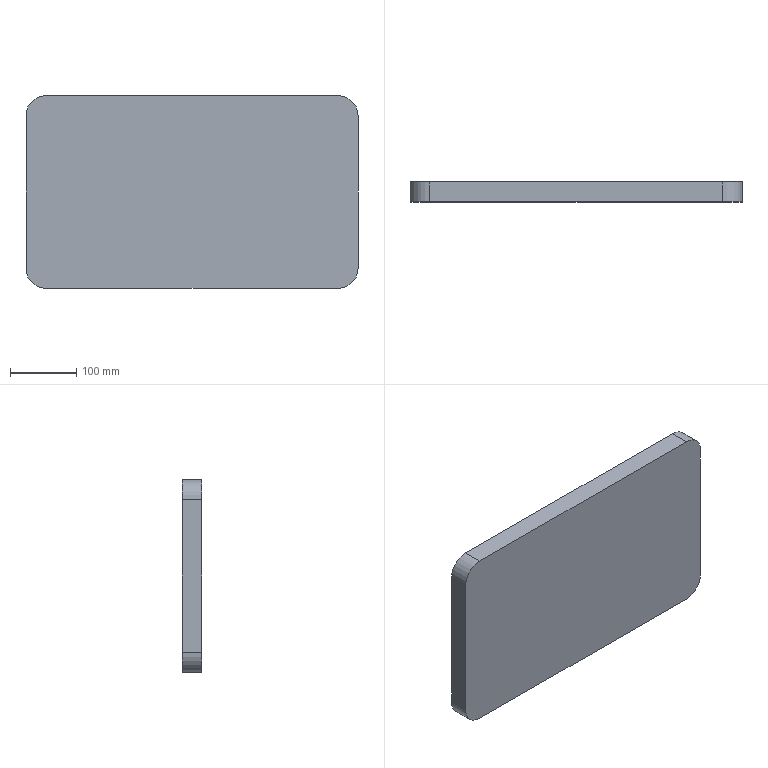Part | SolidWorks | features Extrusion 1, ICE 1 | 1 solid | 19 faces | box 500 x 30 x 290 mm | volume 838737 mm3 | plane 11 | cylinder 8 | commonest cylinder face diameters 60 x8
STEP:
#1=CARTESIAN_POINT('',(250.,0.,-115.));
#2=VERTEX_POINT('',#1);
#3=CARTESIAN_POINT('',(220.,0.,-145.));
#4=VERTEX_POINT('',#3);
#5=CARTESIAN_POINT('',(220.,0.,-115.));
#6=DIRECTION('',(0.,1.,0.));
#7=DIRECTION('',(0.,0.,1.));
#8=AXIS2_PLACEMENT_3D('',#5,#6,#7);
#9=CIRCLE('',#8,30.);
#10=EDGE_CURVE('',#2,#4,#9,.T.);
#11=ORIENTED_EDGE('',*,*,#10,.T.);
#12=CARTESIAN_POINT('',(220.,30.,-145.));
#13=VERTEX_POINT('',#12);
#14=CARTESIAN_POINT('',(220.,30.,-145.));
#15=DIRECTION('',(0.,-1.,0.));
#16=VECTOR('',#15,1000.);
#17=LINE('',#14,#16);
#18=EDGE_CURVE('',#13,#4,#17,.T.);
#19=ORIENTED_EDGE('',*,*,#18,.F.);
#20=CARTESIAN_POINT('',(250.,30.,-115.));
#21=VERTEX_POINT('',#20);
#22=CARTESIAN_POINT('',(220.,30.,-115.));
#23=DIRECTION('',(0.,1.,0.));
#24=DIRECTION('',(0.,0.,1.));
#25=AXIS2_PLACEMENT_3D('',#22,#23,#24);
#26=CIRCLE('',#25,30.);
#27=EDGE_CURVE('',#21,#13,#26,.T.);
#28=ORIENTED_EDGE('',*,*,#27,.F.);
#29=CARTESIAN_POINT('',(250.,30.,-115.));
#30=DIRECTION('',(0.,-1.,0.));
#31=VECTOR('',#30,1000.);
#32=LINE('',#29,#31);
#33=EDGE_CURVE('',#21,#2,#32,.T.);
#34=ORIENTED_EDGE('',*,*,#33,.T.);
#35=EDGE_LOOP('',(#11,#19,#28,#34));
#36=FACE_OUTER_BOUND('',#35,.T.);
#37=CARTESIAN_POINT('',(220.,30.,-115.));
#38=DIRECTION('',(0.,-1.,0.));
#39=DIRECTION('',(0.,0.,-1.));
#40=AXIS2_PLACEMENT_3D('',#37,#38,#39);
#41=CYLINDRICAL_SURFACE('',#40,30.);
#42=ADVANCED_FACE('',(#36),#41,.T.);
#43=CARTESIAN_POINT('',(-220.,0.,-145.));
#44=VERTEX_POINT('',#43);
#45=CARTESIAN_POINT('',(-220.,0.,-145.));
#46=DIRECTION('',(-1.,0.,0.));
#47=VECTOR('',#46,1000.);
#48=LINE('',#45,#47);
#49=EDGE_CURVE('',#4,#44,#48,.T.);
#50=ORIENTED_EDGE('',*,*,#49,.T.);
#51=CARTESIAN_POINT('',(-220.,30.,-145.));
#52=VERTEX_POINT('',#51);
#53=CARTESIAN_POINT('',(-220.,30.,-145.));
#54=DIRECTION('',(0.,-1.,0.));
#55=VECTOR('',#54,1000.);
#56=LINE('',#53,#55);
#57=EDGE_CURVE('',#52,#44,#56,.T.);
#58=ORIENTED_EDGE('',*,*,#57,.F.);
#59=CARTESIAN_POINT('',(-220.,30.,-145.));
#60=DIRECTION('',(-1.,0.,0.));
#61=VECTOR('',#60,1000.);
#62=LINE('',#59,#61);
#63=EDGE_CURVE('',#13,#52,#62,.T.);
#64=ORIENTED_EDGE('',*,*,#63,.F.);
#65=ORIENTED_EDGE('',*,*,#18,.T.);
#66=EDGE_LOOP('',(#50,#58,#64,#65));
#67=FACE_OUTER_BOUND('',#66,.T.);
#68=CARTESIAN_POINT('',(-220.,30.,-145.));
#69=DIRECTION('',(0.,0.,1.));
#70=DIRECTION('',(1.,0.,0.));
#71=AXIS2_PLACEMENT_3D('',#68,#69,#70);
#72=PLANE('',#71);
#73=ADVANCED_FACE('',(#67),#72,.F.);
#74=CARTESIAN_POINT('',(-250.,0.,-115.));
#75=VERTEX_POINT('',#74);
#76=CARTESIAN_POINT('',(-220.,0.,-115.));
#77=DIRECTION('',(0.,1.,0.));
#78=DIRECTION('',(0.,0.,-1.));
#79=AXIS2_PLACEMENT_3D('',#76,#77,#78);
#80=CIRCLE('',#79,30.);
#81=EDGE_CURVE('',#44,#75,#80,.T.);
#82=ORIENTED_EDGE('',*,*,#81,.T.);
#83=CARTESIAN_POINT('',(-250.,30.,-115.));
#84=VERTEX_POINT('',#83);
#85=CARTESIAN_POINT('',(-250.,30.,-115.));
#86=DIRECTION('',(0.,-1.,0.));
#87=VECTOR('',#86,1000.);
#88=LINE('',#85,#87);
#89=EDGE_CURVE('',#84,#75,#88,.T.);
#90=ORIENTED_EDGE('',*,*,#89,.F.);
#91=CARTESIAN_POINT('',(-220.,30.,-115.));
#92=DIRECTION('',(0.,1.,0.));
#93=DIRECTION('',(0.,0.,-1.));
#94=AXIS2_PLACEMENT_3D('',#91,#92,#93);
#95=CIRCLE('',#94,30.);
#96=EDGE_CURVE('',#52,#84,#95,.T.);
#97=ORIENTED_EDGE('',*,*,#96,.F.);
#98=ORIENTED_EDGE('',*,*,#57,.T.);
#99=EDGE_LOOP('',(#82,#90,#97,#98));
#100=FACE_OUTER_BOUND('',#99,.T.);
#101=CARTESIAN_POINT('',(-220.,30.,-115.));
#102=DIRECTION('',(0.,-1.,0.));
#103=DIRECTION('',(0.,0.,-1.));
#104=AXIS2_PLACEMENT_3D('',#101,#102,#103);
#105=CYLINDRICAL_SURFACE('',#104,30.);
#106=ADVANCED_FACE('',(#100),#105,.T.);
#107=CARTESIAN_POINT('',(-250.,0.,115.));
#108=VERTEX_POINT('',#107);
#109=CARTESIAN_POINT('',(-250.,0.,-115.));
#110=DIRECTION('',(0.,0.,1.));
#111=VECTOR('',#110,1000.);
#112=LINE('',#109,#111);
#113=EDGE_CURVE('',#75,#108,#112,.T.);
#114=ORIENTED_EDGE('',*,*,#113,.T.);
#115=CARTESIAN_POINT('',(-250.,30.,115.));
#116=VERTEX_POINT('',#115);
#117=CARTESIAN_POINT('',(-250.,30.,115.));
#118=DIRECTION('',(0.,-1.,0.));
#119=VECTOR('',#118,1000.);
#120=LINE('',#117,#119);
#121=EDGE_CURVE('',#116,#108,#120,.T.);
#122=ORIENTED_EDGE('',*,*,#121,.F.);
#123=CARTESIAN_POINT('',(-250.,30.,-115.));
#124=DIRECTION('',(0.,0.,1.));
#125=VECTOR('',#124,1000.);
#126=LINE('',#123,#125);
#127=EDGE_CURVE('',#84,#116,#126,.T.);
#128=ORIENTED_EDGE('',*,*,#127,.F.);
#129=ORIENTED_EDGE('',*,*,#89,.T.);
#130=EDGE_LOOP('',(#114,#122,#128,#129));
#131=FACE_OUTER_BOUND('',#130,.T.);
#132=CARTESIAN_POINT('',(-250.,30.,-115.));
#133=DIRECTION('',(1.,0.,0.));
#134=DIRECTION('',(0.,0.,-1.));
#135=AXIS2_PLACEMENT_3D('',#132,#133,#134);
#136=PLANE('',#135);
#137=ADVANCED_FACE('',(#131),#136,.F.);
#138=CARTESIAN_POINT('',(-220.,0.,145.));
#139=VERTEX_POINT('',#138);
#140=CARTESIAN_POINT('',(-220.,0.,115.));
#141=DIRECTION('',(0.,1.,0.));
#142=DIRECTION('',(0.,0.,-1.));
#143=AXIS2_PLACEMENT_3D('',#140,#141,#142);
#144=CIRCLE('',#143,30.);
#145=EDGE_CURVE('',#108,#139,#144,.T.);
#146=ORIENTED_EDGE('',*,*,#145,.T.);
#147=CARTESIAN_POINT('',(-220.,30.,145.));
#148=VERTEX_POINT('',#147);
#149=CARTESIAN_POINT('',(-220.,30.,145.));
#150=DIRECTION('',(0.,-1.,0.));
#151=VECTOR('',#150,1000.);
#152=LINE('',#149,#151);
#153=EDGE_CURVE('',#148,#139,#152,.T.);
#154=ORIENTED_EDGE('',*,*,#153,.F.);
#155=CARTESIAN_POINT('',(-220.,30.,115.));
#156=DIRECTION('',(0.,1.,0.));
#157=DIRECTION('',(0.,0.,-1.));
#158=AXIS2_PLACEMENT_3D('',#155,#156,#157);
#159=CIRCLE('',#158,30.);
#160=EDGE_CURVE('',#116,#148,#159,.T.);
#161=ORIENTED_EDGE('',*,*,#160,.F.);
#162=ORIENTED_EDGE('',*,*,#121,.T.);
#163=EDGE_LOOP('',(#146,#154,#161,#162));
#164=FACE_OUTER_BOUND('',#163,.T.);
#165=CARTESIAN_POINT('',(-220.,30.,115.));
#166=DIRECTION('',(0.,-1.,0.));
#167=DIRECTION('',(0.,0.,-1.));
#168=AXIS2_PLACEMENT_3D('',#165,#166,#167);
#169=CYLINDRICAL_SURFACE('',#168,30.);
#170=ADVANCED_FACE('',(#164),#169,.T.);
#171=CARTESIAN_POINT('',(220.,0.,145.));
#172=VERTEX_POINT('',#171);
#173=CARTESIAN_POINT('',(-220.,0.,145.));
#174=DIRECTION('',(1.,0.,0.));
#175=VECTOR('',#174,1000.);
#176=LINE('',#173,#175);
#177=EDGE_CURVE('',#139,#172,#176,.T.);
#178=ORIENTED_EDGE('',*,*,#177,.T.);
#179=CARTESIAN_POINT('',(220.,30.,145.));
#180=VERTEX_POINT('',#179);
#181=CARTESIAN_POINT('',(220.,30.,145.));
#182=DIRECTION('',(0.,-1.,0.));
#183=VECTOR('',#182,1000.);
#184=LINE('',#181,#183);
#185=EDGE_CURVE('',#180,#172,#184,.T.);
#186=ORIENTED_EDGE('',*,*,#185,.F.);
#187=CARTESIAN_POINT('',(-220.,30.,145.));
#188=DIRECTION('',(1.,0.,0.));
#189=VECTOR('',#188,1000.);
#190=LINE('',#187,#189);
#191=EDGE_CURVE('',#148,#180,#190,.T.);
#192=ORIENTED_EDGE('',*,*,#191,.F.);
#193=ORIENTED_EDGE('',*,*,#153,.T.);
#194=EDGE_LOOP('',(#178,#186,#192,#193));
#195=FACE_OUTER_BOUND('',#194,.T.);
#196=CARTESIAN_POINT('',(-220.,30.,145.));
#197=DIRECTION('',(0.,0.,-1.));
#198=DIRECTION('',(-1.,0.,0.));
#199=AXIS2_PLACEMENT_3D('',#196,#197,#198);
#200=PLANE('',#199);
#201=ADVANCED_FACE('',(#195),#200,.F.);
#202=CARTESIAN_POINT('',(250.,0.,115.));
#203=VERTEX_POINT('',#202);
#204=CARTESIAN_POINT('',(220.,0.,115.));
#205=DIRECTION('',(0.,1.,0.));
#206=DIRECTION('',(0.,0.,1.));
#207=AXIS2_PLACEMENT_3D('',#204,#205,#206);
#208=CIRCLE('',#207,30.);
#209=EDGE_CURVE('',#172,#203,#208,.T.);
#210=ORIENTED_EDGE('',*,*,#209,.T.);
#211=CARTESIAN_POINT('',(250.,30.,115.));
#212=VERTEX_POINT('',#211);
#213=CARTESIAN_POINT('',(250.,30.,115.));
#214=DIRECTION('',(0.,-1.,0.));
#215=VECTOR('',#214,1000.);
#216=LINE('',#213,#215);
#217=EDGE_CURVE('',#212,#203,#216,.T.);
#218=ORIENTED_EDGE('',*,*,#217,.F.);
#219=CARTESIAN_POINT('',(220.,30.,115.));
#220=DIRECTION('',(0.,1.,0.));
#221=DIRECTION('',(0.,0.,1.));
#222=AXIS2_PLACEMENT_3D('',#219,#220,#221);
#223=CIRCLE('',#222,30.);
#224=EDGE_CURVE('',#180,#212,#223,.T.);
#225=ORIENTED_EDGE('',*,*,#224,.F.);
#226=ORIENTED_EDGE('',*,*,#185,.T.);
#227=EDGE_LOOP('',(#210,#218,#225,#226));
#228=FACE_OUTER_BOUND('',#227,.T.);
#229=CARTESIAN_POINT('',(220.,30.,115.));
#230=DIRECTION('',(0.,-1.,0.));
#231=DIRECTION('',(0.,0.,-1.));
#232=AXIS2_PLACEMENT_3D('',#229,#230,#231);
#233=CYLINDRICAL_SURFACE('',#232,30.);
#234=ADVANCED_FACE('',(#228),#233,.T.);
#235=CARTESIAN_POINT('',(250.,0.,-115.));
#236=DIRECTION('',(0.,0.,-1.));
#237=VECTOR('',#236,1000.);
#238=LINE('',#235,#237);
#239=EDGE_CURVE('',#203,#2,#238,.T.);
#240=ORIENTED_EDGE('',*,*,#239,.T.);
#241=ORIENTED_EDGE('',*,*,#33,.F.);
#242=CARTESIAN_POINT('',(250.,30.,-115.));
#243=DIRECTION('',(0.,0.,-1.));
#244=VECTOR('',#243,1000.);
#245=LINE('',#242,#244);
#246=EDGE_CURVE('',#212,#21,#245,.T.);
#247=ORIENTED_EDGE('',*,*,#246,.F.);
#248=ORIENTED_EDGE('',*,*,#217,.T.);
#249=EDGE_LOOP('',(#240,#241,#247,#248));
#250=FACE_OUTER_BOUND('',#249,.T.);
#251=CARTESIAN_POINT('',(250.,30.,-115.));
#252=DIRECTION('',(-1.,0.,0.));
#253=DIRECTION('',(0.,0.,1.));
#254=AXIS2_PLACEMENT_3D('',#251,#252,#253);
#255=PLANE('',#254);
#256=ADVANCED_FACE('',(#250),#255,.F.);
#257=CARTESIAN_POINT('',(217.,30.,142.));
#258=VERTEX_POINT('',#257);
#259=CARTESIAN_POINT('',(247.,30.,112.));
#260=VERTEX_POINT('',#259);
#261=CARTESIAN_POINT('',(217.,30.,112.));
#262=DIRECTION('',(0.,1.,0.));
#263=DIRECTION('',(0.,0.,-1.));
#264=AXIS2_PLACEMENT_3D('',#261,#262,#263);
#265=CIRCLE('',#264,30.);
#266=EDGE_CURVE('',#258,#260,#265,.T.);
#267=ORIENTED_EDGE('',*,*,#266,.F.);
#268=CARTESIAN_POINT('',(-217.,30.,142.));
#269=VERTEX_POINT('',#268);
#270=CARTESIAN_POINT('',(-217.,30.,142.));
#271=DIRECTION('',(1.,0.,0.));
#272=VECTOR('',#271,1000.);
#273=LINE('',#270,#272);
#274=EDGE_CURVE('',#269,#258,#273,.T.);
#275=ORIENTED_EDGE('',*,*,#274,.F.);
#276=CARTESIAN_POINT('',(-247.,30.,112.));
#277=VERTEX_POINT('',#276);
#278=CARTESIAN_POINT('',(-217.,30.,112.));
#279=DIRECTION('',(0.,1.,0.));
#280=DIRECTION('',(0.,0.,-1.));
#281=AXIS2_PLACEMENT_3D('',#278,#279,#280);
#282=CIRCLE('',#281,30.);
#283=EDGE_CURVE('',#277,#269,#282,.T.);
#284=ORIENTED_EDGE('',*,*,#283,.F.);
#285=CARTESIAN_POINT('',(-247.,30.,-112.));
#286=VERTEX_POINT('',#285);
#287=CARTESIAN_POINT('',(-247.,30.,-112.));
#288=DIRECTION('',(0.,0.,1.));
#289=VECTOR('',#288,1000.);
#290=LINE('',#287,#289);
#291=EDGE_CURVE('',#286,#277,#290,.T.);
#292=ORIENTED_EDGE('',*,*,#291,.F.);
#293=CARTESIAN_POINT('',(-217.,30.,-142.));
#294=VERTEX_POINT('',#293);
#295=CARTESIAN_POINT('',(-217.,30.,-112.));
#296=DIRECTION('',(0.,1.,0.));
#297=DIRECTION('',(0.,0.,1.));
#298=AXIS2_PLACEMENT_3D('',#295,#296,#297);
#299=CIRCLE('',#298,30.);
#300=EDGE_CURVE('',#294,#286,#299,.T.);
#301=ORIENTED_EDGE('',*,*,#300,.F.);
#302=CARTESIAN_POINT('',(217.,30.,-142.));
#303=VERTEX_POINT('',#302);
#304=CARTESIAN_POINT('',(-217.,30.,-142.));
#305=DIRECTION('',(-1.,0.,0.));
#306=VECTOR('',#305,1000.);
#307=LINE('',#304,#306);
#308=EDGE_CURVE('',#303,#294,#307,.T.);
#309=ORIENTED_EDGE('',*,*,#308,.F.);
#310=CARTESIAN_POINT('',(247.,30.,-112.));
#311=VERTEX_POINT('',#310);
#312=CARTESIAN_POINT('',(217.,30.,-112.));
#313=DIRECTION('',(0.,1.,0.));
#314=DIRECTION('',(0.,0.,-1.));
#315=AXIS2_PLACEMENT_3D('',#312,#313,#314);
#316=CIRCLE('',#315,30.);
#317=EDGE_CURVE('',#311,#303,#316,.T.);
#318=ORIENTED_EDGE('',*,*,#317,.F.);
#319=CARTESIAN_POINT('',(247.,30.,-112.));
#320=DIRECTION('',(0.,0.,-1.));
#321=VECTOR('',#320,1000.);
#322=LINE('',#319,#321);
#323=EDGE_CURVE('',#260,#311,#322,.T.);
#324=ORIENTED_EDGE('',*,*,#323,.F.);
#325=EDGE_LOOP('',(#267,#275,#284,#292,#301,#309,#318,#324));
#326=FACE_BOUND('',#325,.T.);
#327=ORIENTED_EDGE('',*,*,#27,.T.);
#328=ORIENTED_EDGE('',*,*,#63,.T.);
#329=ORIENTED_EDGE('',*,*,#96,.T.);
#330=ORIENTED_EDGE('',*,*,#127,.T.);
#331=ORIENTED_EDGE('',*,*,#160,.T.);
#332=ORIENTED_EDGE('',*,*,#191,.T.);
#333=ORIENTED_EDGE('',*,*,#224,.T.);
#334=ORIENTED_EDGE('',*,*,#246,.T.);
#335=EDGE_LOOP('',(#327,#328,#329,#330,#331,#332,#333,#334));
#336=FACE_OUTER_BOUND('',#335,.T.);
#337=CARTESIAN_POINT('',(220.,30.,-115.));
#338=DIRECTION('',(0.,1.,0.));
#339=DIRECTION('',(0.,0.,1.));
#340=AXIS2_PLACEMENT_3D('',#337,#338,#339);
#341=PLANE('',#340);
#342=ADVANCED_FACE('',(#326,#336),#341,.T.);
#343=ORIENTED_EDGE('',*,*,#10,.F.);
#344=ORIENTED_EDGE('',*,*,#239,.F.);
#345=ORIENTED_EDGE('',*,*,#209,.F.);
#346=ORIENTED_EDGE('',*,*,#177,.F.);
#347=ORIENTED_EDGE('',*,*,#145,.F.);
#348=ORIENTED_EDGE('',*,*,#113,.F.);
#349=ORIENTED_EDGE('',*,*,#81,.F.);
#350=ORIENTED_EDGE('',*,*,#49,.F.);
#351=EDGE_LOOP('',(#343,#344,#345,#346,#347,#348,#349,#350));
#352=FACE_OUTER_BOUND('',#351,.T.);
#353=CARTESIAN_POINT('',(220.,0.,-115.));
#354=DIRECTION('',(0.,1.,0.));
#355=DIRECTION('',(0.,0.,1.));
#356=AXIS2_PLACEMENT_3D('',#353,#354,#355);
#357=PLANE('',#356);
#358=ADVANCED_FACE('',(#352),#357,.F.);
#359=ORIENTED_EDGE('',*,*,#266,.T.);
#360=CARTESIAN_POINT('',(247.,5.,112.));
#361=VERTEX_POINT('',#360);
#362=CARTESIAN_POINT('',(247.,5.,112.));
#363=DIRECTION('',(0.,1.,0.));
#364=VECTOR('',#363,1000.);
#365=LINE('',#362,#364);
#366=EDGE_CURVE('',#361,#260,#365,.T.);
#367=ORIENTED_EDGE('',*,*,#366,.F.);
#368=CARTESIAN_POINT('',(217.,5.,142.));
#369=VERTEX_POINT('',#368);
#370=CARTESIAN_POINT('',(217.,5.,112.));
#371=DIRECTION('',(0.,1.,0.));
#372=DIRECTION('',(0.,0.,-1.));
#373=AXIS2_PLACEMENT_3D('',#370,#371,#372);
#374=CIRCLE('',#373,30.);
#375=EDGE_CURVE('',#369,#361,#374,.T.);
#376=ORIENTED_EDGE('',*,*,#375,.F.);
#377=CARTESIAN_POINT('',(217.,5.,142.));
#378=DIRECTION('',(0.,1.,0.));
#379=VECTOR('',#378,1000.);
#380=LINE('',#377,#379);
#381=EDGE_CURVE('',#369,#258,#380,.T.);
#382=ORIENTED_EDGE('',*,*,#381,.T.);
#383=EDGE_LOOP('',(#359,#367,#376,#382));
#384=FACE_OUTER_BOUND('',#383,.T.);
#385=CARTESIAN_POINT('',(217.,5.,112.));
#386=DIRECTION('',(0.,1.,0.));
#387=DIRECTION('',(0.,0.,1.));
#388=AXIS2_PLACEMENT_3D('',#385,#386,#387);
#389=CYLINDRICAL_SURFACE('',#388,30.);
#390=ADVANCED_FACE('',(#384),#389,.F.);
#391=ORIENTED_EDGE('',*,*,#274,.T.);
#392=ORIENTED_EDGE('',*,*,#381,.F.);
#393=CARTESIAN_POINT('',(-217.,5.,142.));
#394=VERTEX_POINT('',#393);
#395=CARTESIAN_POINT('',(-217.,5.,142.));
#396=DIRECTION('',(1.,0.,0.));
#397=VECTOR('',#396,1000.);
#398=LINE('',#395,#397);
#399=EDGE_CURVE('',#394,#369,#398,.T.);
#400=ORIENTED_EDGE('',*,*,#399,.F.);
#401=CARTESIAN_POINT('',(-217.,5.,142.));
#402=DIRECTION('',(0.,1.,0.));
#403=VECTOR('',#402,1000.);
#404=LINE('',#401,#403);
#405=EDGE_CURVE('',#394,#269,#404,.T.);
#406=ORIENTED_EDGE('',*,*,#405,.T.);
#407=EDGE_LOOP('',(#391,#392,#400,#406));
#408=FACE_OUTER_BOUND('',#407,.T.);
#409=CARTESIAN_POINT('',(-217.,5.,142.));
#410=DIRECTION('',(0.,0.,1.));
#411=DIRECTION('',(1.,0.,0.));
#412=AXIS2_PLACEMENT_3D('',#409,#410,#411);
#413=PLANE('',#412);
#414=ADVANCED_FACE('',(#408),#413,.F.);
#415=ORIENTED_EDGE('',*,*,#283,.T.);
#416=ORIENTED_EDGE('',*,*,#405,.F.);
#417=CARTESIAN_POINT('',(-247.,5.,112.));
#418=VERTEX_POINT('',#417);
#419=CARTESIAN_POINT('',(-217.,5.,112.));
#420=DIRECTION('',(0.,1.,0.));
#421=DIRECTION('',(0.,0.,-1.));
#422=AXIS2_PLACEMENT_3D('',#419,#420,#421);
#423=CIRCLE('',#422,30.);
#424=EDGE_CURVE('',#418,#394,#423,.T.);
#425=ORIENTED_EDGE('',*,*,#424,.F.);
#426=CARTESIAN_POINT('',(-247.,5.,112.));
#427=DIRECTION('',(0.,1.,0.));
#428=VECTOR('',#427,1000.);
#429=LINE('',#426,#428);
#430=EDGE_CURVE('',#418,#277,#429,.T.);
#431=ORIENTED_EDGE('',*,*,#430,.T.);
#432=EDGE_LOOP('',(#415,#416,#425,#431));
#433=FACE_OUTER_BOUND('',#432,.T.);
#434=CARTESIAN_POINT('',(-217.,5.,112.));
#435=DIRECTION('',(0.,1.,0.));
#436=DIRECTION('',(0.,0.,1.));
#437=AXIS2_PLACEMENT_3D('',#434,#435,#436);
#438=CYLINDRICAL_SURFACE('',#437,30.);
#439=ADVANCED_FACE('',(#433),#438,.F.);
#440=ORIENTED_EDGE('',*,*,#291,.T.);
#441=ORIENTED_EDGE('',*,*,#430,.F.);
#442=CARTESIAN_POINT('',(-247.,5.,-112.));
#443=VERTEX_POINT('',#442);
#444=CARTESIAN_POINT('',(-247.,5.,-112.));
#445=DIRECTION('',(0.,0.,1.));
#446=VECTOR('',#445,1000.);
#447=LINE('',#444,#446);
#448=EDGE_CURVE('',#443,#418,#447,.T.);
#449=ORIENTED_EDGE('',*,*,#448,.F.);
#450=CARTESIAN_POINT('',(-247.,5.,-112.));
#451=DIRECTION('',(0.,1.,0.));
#452=VECTOR('',#451,1000.);
#453=LINE('',#450,#452);
#454=EDGE_CURVE('',#443,#286,#453,.T.);
#455=ORIENTED_EDGE('',*,*,#454,.T.);
#456=EDGE_LOOP('',(#440,#441,#449,#455));
#457=FACE_OUTER_BOUND('',#456,.T.);
#458=CARTESIAN_POINT('',(-247.,5.,-112.));
#459=DIRECTION('',(-1.,0.,0.));
#460=DIRECTION('',(0.,0.,1.));
#461=AXIS2_PLACEMENT_3D('',#458,#459,#460);
#462=PLANE('',#461);
#463=ADVANCED_FACE('',(#457),#462,.F.);
#464=ORIENTED_EDGE('',*,*,#300,.T.);
#465=ORIENTED_EDGE('',*,*,#454,.F.);
#466=CARTESIAN_POINT('',(-217.,5.,-142.));
#467=VERTEX_POINT('',#466);
#468=CARTESIAN_POINT('',(-217.,5.,-112.));
#469=DIRECTION('',(0.,1.,0.));
#470=DIRECTION('',(0.,0.,1.));
#471=AXIS2_PLACEMENT_3D('',#468,#469,#470);
#472=CIRCLE('',#471,30.);
#473=EDGE_CURVE('',#467,#443,#472,.T.);
#474=ORIENTED_EDGE('',*,*,#473,.F.);
#475=CARTESIAN_POINT('',(-217.,5.,-142.));
#476=DIRECTION('',(0.,1.,0.));
#477=VECTOR('',#476,1000.);
#478=LINE('',#475,#477);
#479=EDGE_CURVE('',#467,#294,#478,.T.);
#480=ORIENTED_EDGE('',*,*,#479,.T.);
#481=EDGE_LOOP('',(#464,#465,#474,#480));
#482=FACE_OUTER_BOUND('',#481,.T.);
#483=CARTESIAN_POINT('',(-217.,5.,-112.));
#484=DIRECTION('',(0.,1.,0.));
#485=DIRECTION('',(0.,0.,1.));
#486=AXIS2_PLACEMENT_3D('',#483,#484,#485);
#487=CYLINDRICAL_SURFACE('',#486,30.);
#488=ADVANCED_FACE('',(#482),#487,.F.);
#489=ORIENTED_EDGE('',*,*,#308,.T.);
#490=ORIENTED_EDGE('',*,*,#479,.F.);
#491=CARTESIAN_POINT('',(217.,5.,-142.));
#492=VERTEX_POINT('',#491);
#493=CARTESIAN_POINT('',(-217.,5.,-142.));
#494=DIRECTION('',(-1.,0.,0.));
#495=VECTOR('',#494,1000.);
#496=LINE('',#493,#495);
#497=EDGE_CURVE('',#492,#467,#496,.T.);
#498=ORIENTED_EDGE('',*,*,#497,.F.);
#499=CARTESIAN_POINT('',(217.,5.,-142.));
#500=DIRECTION('',(0.,1.,0.));
#501=VECTOR('',#500,1000.);
#502=LINE('',#499,#501);
#503=EDGE_CURVE('',#492,#303,#502,.T.);
#504=ORIENTED_EDGE('',*,*,#503,.T.);
#505=EDGE_LOOP('',(#489,#490,#498,#504));
#506=FACE_OUTER_BOUND('',#505,.T.);
#507=CARTESIAN_POINT('',(-217.,5.,-142.));
#508=DIRECTION('',(0.,0.,-1.));
#509=DIRECTION('',(-1.,0.,0.));
#510=AXIS2_PLACEMENT_3D('',#507,#508,#509);
#511=PLANE('',#510);
#512=ADVANCED_FACE('',(#506),#511,.F.);
#513=ORIENTED_EDGE('',*,*,#317,.T.);
#514=ORIENTED_EDGE('',*,*,#503,.F.);
#515=CARTESIAN_POINT('',(247.,5.,-112.));
#516=VERTEX_POINT('',#515);
#517=CARTESIAN_POINT('',(217.,5.,-112.));
#518=DIRECTION('',(0.,1.,0.));
#519=DIRECTION('',(0.,0.,-1.));
#520=AXIS2_PLACEMENT_3D('',#517,#518,#519);
#521=CIRCLE('',#520,30.);
#522=EDGE_CURVE('',#516,#492,#521,.T.);
#523=ORIENTED_EDGE('',*,*,#522,.F.);
#524=CARTESIAN_POINT('',(247.,5.,-112.));
#525=DIRECTION('',(0.,1.,0.));
#526=VECTOR('',#525,1000.);
#527=LINE('',#524,#526);
#528=EDGE_CURVE('',#516,#311,#527,.T.);
#529=ORIENTED_EDGE('',*,*,#528,.T.);
#530=EDGE_LOOP('',(#513,#514,#523,#529));
#531=FACE_OUTER_BOUND('',#530,.T.);
#532=CARTESIAN_POINT('',(217.,5.,-112.));
#533=DIRECTION('',(0.,1.,0.));
#534=DIRECTION('',(0.,0.,1.));
#535=AXIS2_PLACEMENT_3D('',#532,#533,#534);
#536=CYLINDRICAL_SURFACE('',#535,30.);
#537=ADVANCED_FACE('',(#531),#536,.F.);
#538=ORIENTED_EDGE('',*,*,#323,.T.);
#539=ORIENTED_EDGE('',*,*,#528,.F.);
#540=CARTESIAN_POINT('',(247.,5.,-112.));
#541=DIRECTION('',(0.,0.,-1.));
#542=VECTOR('',#541,1000.);
#543=LINE('',#540,#542);
#544=EDGE_CURVE('',#361,#516,#543,.T.);
#545=ORIENTED_EDGE('',*,*,#544,.F.);
#546=ORIENTED_EDGE('',*,*,#366,.T.);
#547=EDGE_LOOP('',(#538,#539,#545,#546));
#548=FACE_OUTER_BOUND('',#547,.T.);
#549=CARTESIAN_POINT('',(247.,5.,-112.));
#550=DIRECTION('',(1.,0.,0.));
#551=DIRECTION('',(0.,0.,-1.));
#552=AXIS2_PLACEMENT_3D('',#549,#550,#551);
#553=PLANE('',#552);
#554=ADVANCED_FACE('',(#548),#553,.F.);
#555=ORIENTED_EDGE('',*,*,#375,.T.);
#556=ORIENTED_EDGE('',*,*,#544,.T.);
#557=ORIENTED_EDGE('',*,*,#522,.T.);
#558=ORIENTED_EDGE('',*,*,#497,.T.);
#559=ORIENTED_EDGE('',*,*,#473,.T.);
#560=ORIENTED_EDGE('',*,*,#448,.T.);
#561=ORIENTED_EDGE('',*,*,#424,.T.);
#562=ORIENTED_EDGE('',*,*,#399,.T.);
#563=EDGE_LOOP('',(#555,#556,#557,#558,#559,#560,#561,#562));
#564=FACE_OUTER_BOUND('',#563,.T.);
#565=CARTESIAN_POINT('',(217.,5.,112.));
#566=DIRECTION('',(0.,-1.,0.));
#567=DIRECTION('',(0.,0.,-1.));
#568=AXIS2_PLACEMENT_3D('',#565,#566,#567);
#569=PLANE('',#568);
#570=ADVANCED_FACE('',(#564),#569,.F.);
#571=CLOSED_SHELL('',(#42,#73,#106,#137,#170,#201,#234,#256,#342,#358,#390,#414,#439,#463,#488,#512,#537,#554,#570));
#572=MANIFOLD_SOLID_BREP('',#571);
#573=CARTESIAN_POINT('',(0.,0.,0.));
#574=DIRECTION('',(0.,0.,1.));
#575=DIRECTION('',(1.,0.,0.));
#576=AXIS2_PLACEMENT_3D('',#573,#574,#575);
#577=(LENGTH_UNIT()NAMED_UNIT(*)SI_UNIT(.MILLI.,.METRE.));
#578=UNCERTAINTY_MEASURE_WITH_UNIT(LENGTH_MEASURE(0.00001),#577,'','');
#579=(NAMED_UNIT(*)PLANE_ANGLE_UNIT()SI_UNIT($,.RADIAN.));
#580=(NAMED_UNIT(*)SI_UNIT($,.STERADIAN.)SOLID_ANGLE_UNIT());
#581=(GEOMETRIC_REPRESENTATION_CONTEXT(3)GLOBAL_UNCERTAINTY_ASSIGNED_CONTEXT((#578))GLOBAL_UNIT_ASSIGNED_CONTEXT((#577,#579,#580))REPRESENTATION_CONTEXT('',''));
#582=ADVANCED_BREP_SHAPE_REPRESENTATION('',(#572,#576),#581);